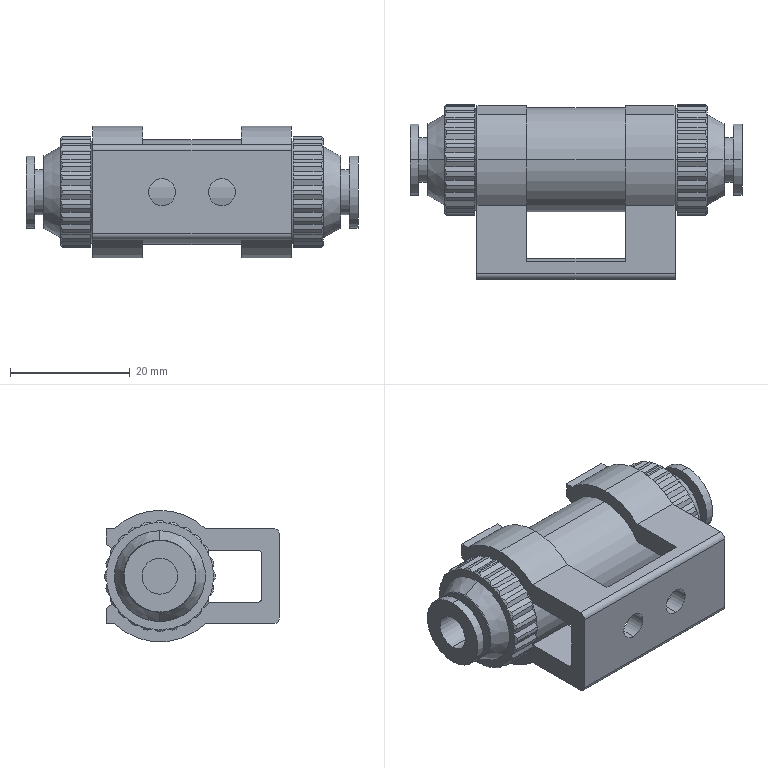Part | STEP file | Vacuum filter Qilike VFD-02-06-1 | 1 solid | 278 faces | box 55.5 x 29.25 x 22 mm | volume 15469 mm3 | plane 138 | cylinder 78 | cone 58 | spline 4 | commonest cylinder face diameters 18.5 x50 22 x6 4.5 x4 6 x4 7.5 x4 12 x4